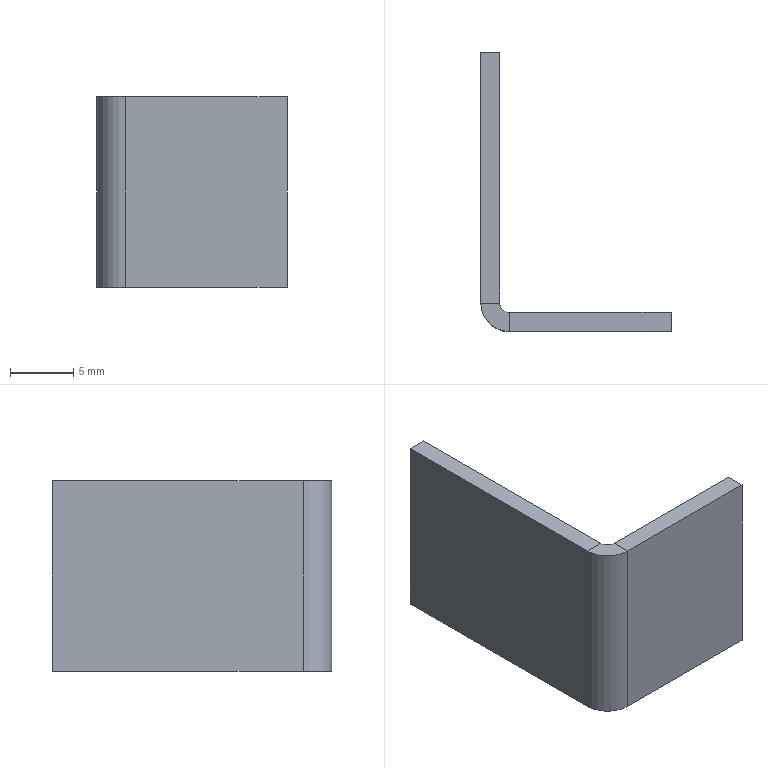Part | SolidWorks | features FlatPattern 1, SMBaseFlange 1, SheetMetal 1 | 1 solid | 14 faces | box 15 x 22 x 15 mm | volume 784.394 mm3 | plane 12 | cylinder 2 | commonest cylinder face diameters 1.473 x1 4.473 x1
STEP:
#1=CARTESIAN_POINT('',(-15.,2.237,7.5));
#2=VERTEX_POINT('',#1);
#3=CARTESIAN_POINT('',(-13.5,2.237,7.5));
#4=VERTEX_POINT('',#3);
#5=CARTESIAN_POINT('',(-15.,2.237,7.5));
#6=DIRECTION('',(1.,0.,0.));
#7=VECTOR('',#6,1000.);
#8=LINE('',#5,#7);
#9=EDGE_CURVE('',#2,#4,#8,.T.);
#10=ORIENTED_EDGE('',*,*,#9,.F.);
#11=CARTESIAN_POINT('',(-12.763,0.,7.5));
#12=VERTEX_POINT('',#11);
#13=CARTESIAN_POINT('',(-12.763,2.237,7.5));
#14=DIRECTION('',(0.,0.,-1.));
#15=DIRECTION('',(1.,0.,0.));
#16=AXIS2_PLACEMENT_3D('',#13,#14,#15);
#17=CIRCLE('',#16,2.237);
#18=EDGE_CURVE('',#12,#2,#17,.T.);
#19=ORIENTED_EDGE('',*,*,#18,.F.);
#20=CARTESIAN_POINT('',(-12.763,1.5,7.5));
#21=VERTEX_POINT('',#20);
#22=CARTESIAN_POINT('',(-12.763,1.5,7.5));
#23=DIRECTION('',(0.,-1.,0.));
#24=VECTOR('',#23,1000.);
#25=LINE('',#22,#24);
#26=EDGE_CURVE('',#21,#12,#25,.T.);
#27=ORIENTED_EDGE('',*,*,#26,.F.);
#28=CARTESIAN_POINT('',(-12.763,2.237,7.5));
#29=DIRECTION('',(0.,0.,-1.));
#30=DIRECTION('',(1.,0.,0.));
#31=AXIS2_PLACEMENT_3D('',#28,#29,#30);
#32=CIRCLE('',#31,0.7366);
#33=EDGE_CURVE('',#21,#4,#32,.T.);
#34=ORIENTED_EDGE('',*,*,#33,.T.);
#35=EDGE_LOOP('',(#10,#19,#27,#34));
#36=FACE_OUTER_BOUND('',#35,.T.);
#37=CARTESIAN_POINT('',(-15.,2.237,7.5));
#38=DIRECTION('',(0.,0.,1.));
#39=DIRECTION('',(1.,0.,0.));
#40=AXIS2_PLACEMENT_3D('',#37,#38,#39);
#41=PLANE('',#40);
#42=ADVANCED_FACE('',(#36),#41,.T.);
#43=CARTESIAN_POINT('',(-15.,22.,7.5));
#44=VERTEX_POINT('',#43);
#45=CARTESIAN_POINT('',(-15.,0.,7.5));
#46=DIRECTION('',(0.,1.,0.));
#47=VECTOR('',#46,1000.);
#48=LINE('',#45,#47);
#49=EDGE_CURVE('',#2,#44,#48,.T.);
#50=ORIENTED_EDGE('',*,*,#49,.F.);
#51=ORIENTED_EDGE('',*,*,#9,.T.);
#52=CARTESIAN_POINT('',(-13.5,22.,7.5));
#53=VERTEX_POINT('',#52);
#54=CARTESIAN_POINT('',(-13.5,0.,7.5));
#55=DIRECTION('',(0.,1.,0.));
#56=VECTOR('',#55,1000.);
#57=LINE('',#54,#56);
#58=EDGE_CURVE('',#4,#53,#57,.T.);
#59=ORIENTED_EDGE('',*,*,#58,.T.);
#60=CARTESIAN_POINT('',(-15.,22.,7.5));
#61=DIRECTION('',(1.,0.,0.));
#62=VECTOR('',#61,1000.);
#63=LINE('',#60,#62);
#64=EDGE_CURVE('',#44,#53,#63,.T.);
#65=ORIENTED_EDGE('',*,*,#64,.F.);
#66=EDGE_LOOP('',(#50,#51,#59,#65));
#67=FACE_OUTER_BOUND('',#66,.T.);
#68=CARTESIAN_POINT('',(-12.763,1.5,7.5));
#69=DIRECTION('',(0.,0.,1.));
#70=DIRECTION('',(1.,0.,0.));
#71=AXIS2_PLACEMENT_3D('',#68,#69,#70);
#72=PLANE('',#71);
#73=ADVANCED_FACE('',(#67),#72,.T.);
#74=CARTESIAN_POINT('',(-12.763,0.,-7.5));
#75=VERTEX_POINT('',#74);
#76=CARTESIAN_POINT('',(-12.763,1.5,-7.5));
#77=VERTEX_POINT('',#76);
#78=CARTESIAN_POINT('',(-12.763,0.,-7.5));
#79=DIRECTION('',(0.,1.,0.));
#80=VECTOR('',#79,1000.);
#81=LINE('',#78,#80);
#82=EDGE_CURVE('',#75,#77,#81,.T.);
#83=ORIENTED_EDGE('',*,*,#82,.F.);
#84=CARTESIAN_POINT('',(-15.,2.237,-7.5));
#85=VERTEX_POINT('',#84);
#86=CARTESIAN_POINT('',(-12.763,2.237,-7.5));
#87=DIRECTION('',(0.,0.,-1.));
#88=DIRECTION('',(1.,0.,0.));
#89=AXIS2_PLACEMENT_3D('',#86,#87,#88);
#90=CIRCLE('',#89,2.237);
#91=EDGE_CURVE('',#75,#85,#90,.T.);
#92=ORIENTED_EDGE('',*,*,#91,.T.);
#93=CARTESIAN_POINT('',(-13.5,2.237,-7.5));
#94=VERTEX_POINT('',#93);
#95=CARTESIAN_POINT('',(-13.5,2.237,-7.5));
#96=DIRECTION('',(-1.,0.,0.));
#97=VECTOR('',#96,1000.);
#98=LINE('',#95,#97);
#99=EDGE_CURVE('',#94,#85,#98,.T.);
#100=ORIENTED_EDGE('',*,*,#99,.F.);
#101=CARTESIAN_POINT('',(-12.763,2.237,-7.5));
#102=DIRECTION('',(0.,0.,-1.));
#103=DIRECTION('',(1.,0.,0.));
#104=AXIS2_PLACEMENT_3D('',#101,#102,#103);
#105=CIRCLE('',#104,0.7366);
#106=EDGE_CURVE('',#77,#94,#105,.T.);
#107=ORIENTED_EDGE('',*,*,#106,.F.);
#108=EDGE_LOOP('',(#83,#92,#100,#107));
#109=FACE_OUTER_BOUND('',#108,.T.);
#110=CARTESIAN_POINT('',(-12.763,0.,-7.5));
#111=DIRECTION('',(0.,0.,-1.));
#112=DIRECTION('',(-1.,0.,0.));
#113=AXIS2_PLACEMENT_3D('',#110,#111,#112);
#114=PLANE('',#113);
#115=ADVANCED_FACE('',(#109),#114,.T.);
#116=CARTESIAN_POINT('',(0.,0.,-7.5));
#117=VERTEX_POINT('',#116);
#118=CARTESIAN_POINT('',(0.,0.,-7.5));
#119=DIRECTION('',(-1.,0.,0.));
#120=VECTOR('',#119,1000.);
#121=LINE('',#118,#120);
#122=EDGE_CURVE('',#117,#75,#121,.T.);
#123=ORIENTED_EDGE('',*,*,#122,.T.);
#124=ORIENTED_EDGE('',*,*,#82,.T.);
#125=CARTESIAN_POINT('',(0.,1.5,-7.5));
#126=VERTEX_POINT('',#125);
#127=CARTESIAN_POINT('',(0.,1.5,-7.5));
#128=DIRECTION('',(-1.,0.,0.));
#129=VECTOR('',#128,1000.);
#130=LINE('',#127,#129);
#131=EDGE_CURVE('',#126,#77,#130,.T.);
#132=ORIENTED_EDGE('',*,*,#131,.F.);
#133=CARTESIAN_POINT('',(0.,1.5,-7.5));
#134=DIRECTION('',(0.,-1.,0.));
#135=VECTOR('',#134,1000.);
#136=LINE('',#133,#135);
#137=EDGE_CURVE('',#126,#117,#136,.T.);
#138=ORIENTED_EDGE('',*,*,#137,.T.);
#139=EDGE_LOOP('',(#123,#124,#132,#138));
#140=FACE_OUTER_BOUND('',#139,.T.);
#141=CARTESIAN_POINT('',(-13.5,2.237,-7.5));
#142=DIRECTION('',(0.,0.,-1.));
#143=DIRECTION('',(-1.,0.,0.));
#144=AXIS2_PLACEMENT_3D('',#141,#142,#143);
#145=PLANE('',#144);
#146=ADVANCED_FACE('',(#140),#145,.T.);
#147=CARTESIAN_POINT('',(-13.5,22.,-7.5));
#148=VERTEX_POINT('',#147);
#149=CARTESIAN_POINT('',(-13.5,0.,-7.5));
#150=DIRECTION('',(0.,1.,0.));
#151=VECTOR('',#150,1000.);
#152=LINE('',#149,#151);
#153=EDGE_CURVE('',#94,#148,#152,.T.);
#154=ORIENTED_EDGE('',*,*,#153,.T.);
#155=CARTESIAN_POINT('',(-13.5,22.,7.5));
#156=DIRECTION('',(0.,0.,-1.));
#157=VECTOR('',#156,1000.);
#158=LINE('',#155,#157);
#159=EDGE_CURVE('',#53,#148,#158,.T.);
#160=ORIENTED_EDGE('',*,*,#159,.F.);
#161=ORIENTED_EDGE('',*,*,#58,.F.);
#162=CARTESIAN_POINT('',(-13.5,2.237,7.5));
#163=DIRECTION('',(0.,0.,-1.));
#164=VECTOR('',#163,1000.);
#165=LINE('',#162,#164);
#166=EDGE_CURVE('',#4,#94,#165,.T.);
#167=ORIENTED_EDGE('',*,*,#166,.T.);
#168=EDGE_LOOP('',(#154,#160,#161,#167));
#169=FACE_OUTER_BOUND('',#168,.T.);
#170=CARTESIAN_POINT('',(-13.5,0.,7.5));
#171=DIRECTION('',(-1.,0.,0.));
#172=DIRECTION('',(0.,0.,1.));
#173=AXIS2_PLACEMENT_3D('',#170,#171,#172);
#174=PLANE('',#173);
#175=ADVANCED_FACE('',(#169),#174,.F.);
#176=CARTESIAN_POINT('',(-15.,22.,-7.5));
#177=VERTEX_POINT('',#176);
#178=CARTESIAN_POINT('',(-15.,22.,-7.5));
#179=DIRECTION('',(1.,0.,0.));
#180=VECTOR('',#179,1000.);
#181=LINE('',#178,#180);
#182=EDGE_CURVE('',#177,#148,#181,.T.);
#183=ORIENTED_EDGE('',*,*,#182,.F.);
#184=CARTESIAN_POINT('',(-15.,22.,7.5));
#185=DIRECTION('',(0.,0.,-1.));
#186=VECTOR('',#185,1000.);
#187=LINE('',#184,#186);
#188=EDGE_CURVE('',#44,#177,#187,.T.);
#189=ORIENTED_EDGE('',*,*,#188,.F.);
#190=ORIENTED_EDGE('',*,*,#64,.T.);
#191=ORIENTED_EDGE('',*,*,#159,.T.);
#192=EDGE_LOOP('',(#183,#189,#190,#191));
#193=FACE_OUTER_BOUND('',#192,.T.);
#194=CARTESIAN_POINT('',(-15.,22.,7.5));
#195=DIRECTION('',(0.,1.,0.));
#196=DIRECTION('',(0.,0.,1.));
#197=AXIS2_PLACEMENT_3D('',#194,#195,#196);
#198=PLANE('',#197);
#199=ADVANCED_FACE('',(#193),#198,.T.);
#200=CARTESIAN_POINT('',(-15.,0.,-7.5));
#201=DIRECTION('',(0.,1.,0.));
#202=VECTOR('',#201,1000.);
#203=LINE('',#200,#202);
#204=EDGE_CURVE('',#85,#177,#203,.T.);
#205=ORIENTED_EDGE('',*,*,#204,.F.);
#206=CARTESIAN_POINT('',(-15.,2.237,7.5));
#207=DIRECTION('',(0.,0.,-1.));
#208=VECTOR('',#207,1000.);
#209=LINE('',#206,#208);
#210=EDGE_CURVE('',#2,#85,#209,.T.);
#211=ORIENTED_EDGE('',*,*,#210,.F.);
#212=ORIENTED_EDGE('',*,*,#49,.T.);
#213=ORIENTED_EDGE('',*,*,#188,.T.);
#214=EDGE_LOOP('',(#205,#211,#212,#213));
#215=FACE_OUTER_BOUND('',#214,.T.);
#216=CARTESIAN_POINT('',(-15.,0.,7.5));
#217=DIRECTION('',(-1.,0.,0.));
#218=DIRECTION('',(0.,0.,1.));
#219=AXIS2_PLACEMENT_3D('',#216,#217,#218);
#220=PLANE('',#219);
#221=ADVANCED_FACE('',(#215),#220,.T.);
#222=ORIENTED_EDGE('',*,*,#91,.F.);
#223=CARTESIAN_POINT('',(-12.763,0.,7.5));
#224=DIRECTION('',(0.,0.,-1.));
#225=VECTOR('',#224,1000.);
#226=LINE('',#223,#225);
#227=EDGE_CURVE('',#12,#75,#226,.T.);
#228=ORIENTED_EDGE('',*,*,#227,.F.);
#229=ORIENTED_EDGE('',*,*,#18,.T.);
#230=ORIENTED_EDGE('',*,*,#210,.T.);
#231=EDGE_LOOP('',(#222,#228,#229,#230));
#232=FACE_OUTER_BOUND('',#231,.T.);
#233=CARTESIAN_POINT('',(-12.763,2.237,7.5));
#234=DIRECTION('',(0.,0.,-1.));
#235=DIRECTION('',(-1.,0.,0.));
#236=AXIS2_PLACEMENT_3D('',#233,#234,#235);
#237=CYLINDRICAL_SURFACE('',#236,2.237);
#238=ADVANCED_FACE('',(#232),#237,.T.);
#239=ORIENTED_EDGE('',*,*,#122,.F.);
#240=CARTESIAN_POINT('',(0.,0.,7.5));
#241=VERTEX_POINT('',#240);
#242=CARTESIAN_POINT('',(0.,0.,7.5));
#243=DIRECTION('',(0.,0.,-1.));
#244=VECTOR('',#243,1000.);
#245=LINE('',#242,#244);
#246=EDGE_CURVE('',#241,#117,#245,.T.);
#247=ORIENTED_EDGE('',*,*,#246,.F.);
#248=CARTESIAN_POINT('',(0.,0.,7.5));
#249=DIRECTION('',(-1.,0.,0.));
#250=VECTOR('',#249,1000.);
#251=LINE('',#248,#250);
#252=EDGE_CURVE('',#241,#12,#251,.T.);
#253=ORIENTED_EDGE('',*,*,#252,.T.);
#254=ORIENTED_EDGE('',*,*,#227,.T.);
#255=EDGE_LOOP('',(#239,#247,#253,#254));
#256=FACE_OUTER_BOUND('',#255,.T.);
#257=CARTESIAN_POINT('',(0.,0.,7.5));
#258=DIRECTION('',(0.,-1.,0.));
#259=DIRECTION('',(0.,0.,-1.));
#260=AXIS2_PLACEMENT_3D('',#257,#258,#259);
#261=PLANE('',#260);
#262=ADVANCED_FACE('',(#256),#261,.T.);
#263=ORIENTED_EDGE('',*,*,#137,.F.);
#264=CARTESIAN_POINT('',(0.,1.5,7.5));
#265=VERTEX_POINT('',#264);
#266=CARTESIAN_POINT('',(0.,1.5,7.5));
#267=DIRECTION('',(0.,0.,-1.));
#268=VECTOR('',#267,1000.);
#269=LINE('',#266,#268);
#270=EDGE_CURVE('',#265,#126,#269,.T.);
#271=ORIENTED_EDGE('',*,*,#270,.F.);
#272=CARTESIAN_POINT('',(0.,1.5,7.5));
#273=DIRECTION('',(0.,-1.,0.));
#274=VECTOR('',#273,1000.);
#275=LINE('',#272,#274);
#276=EDGE_CURVE('',#265,#241,#275,.T.);
#277=ORIENTED_EDGE('',*,*,#276,.T.);
#278=ORIENTED_EDGE('',*,*,#246,.T.);
#279=EDGE_LOOP('',(#263,#271,#277,#278));
#280=FACE_OUTER_BOUND('',#279,.T.);
#281=CARTESIAN_POINT('',(0.,1.5,7.5));
#282=DIRECTION('',(1.,0.,0.));
#283=DIRECTION('',(0.,0.,-1.));
#284=AXIS2_PLACEMENT_3D('',#281,#282,#283);
#285=PLANE('',#284);
#286=ADVANCED_FACE('',(#280),#285,.T.);
#287=ORIENTED_EDGE('',*,*,#131,.T.);
#288=CARTESIAN_POINT('',(-12.763,1.5,7.5));
#289=DIRECTION('',(0.,0.,-1.));
#290=VECTOR('',#289,1000.);
#291=LINE('',#288,#290);
#292=EDGE_CURVE('',#21,#77,#291,.T.);
#293=ORIENTED_EDGE('',*,*,#292,.F.);
#294=CARTESIAN_POINT('',(0.,1.5,7.5));
#295=DIRECTION('',(-1.,0.,0.));
#296=VECTOR('',#295,1000.);
#297=LINE('',#294,#296);
#298=EDGE_CURVE('',#265,#21,#297,.T.);
#299=ORIENTED_EDGE('',*,*,#298,.F.);
#300=ORIENTED_EDGE('',*,*,#270,.T.);
#301=EDGE_LOOP('',(#287,#293,#299,#300));
#302=FACE_OUTER_BOUND('',#301,.T.);
#303=CARTESIAN_POINT('',(0.,1.5,7.5));
#304=DIRECTION('',(0.,-1.,0.));
#305=DIRECTION('',(0.,0.,-1.));
#306=AXIS2_PLACEMENT_3D('',#303,#304,#305);
#307=PLANE('',#306);
#308=ADVANCED_FACE('',(#302),#307,.F.);
#309=ORIENTED_EDGE('',*,*,#106,.T.);
#310=ORIENTED_EDGE('',*,*,#166,.F.);
#311=ORIENTED_EDGE('',*,*,#33,.F.);
#312=ORIENTED_EDGE('',*,*,#292,.T.);
#313=EDGE_LOOP('',(#309,#310,#311,#312));
#314=FACE_OUTER_BOUND('',#313,.T.);
#315=CARTESIAN_POINT('',(-12.763,2.237,7.5));
#316=DIRECTION('',(0.,0.,-1.));
#317=DIRECTION('',(-1.,0.,0.));
#318=AXIS2_PLACEMENT_3D('',#315,#316,#317);
#319=CYLINDRICAL_SURFACE('',#318,0.7366);
#320=ADVANCED_FACE('',(#314),#319,.F.);
#321=ORIENTED_EDGE('',*,*,#298,.T.);
#322=ORIENTED_EDGE('',*,*,#26,.T.);
#323=ORIENTED_EDGE('',*,*,#252,.F.);
#324=ORIENTED_EDGE('',*,*,#276,.F.);
#325=EDGE_LOOP('',(#321,#322,#323,#324));
#326=FACE_OUTER_BOUND('',#325,.T.);
#327=CARTESIAN_POINT('',(-12.763,2.237,7.5));
#328=DIRECTION('',(0.,0.,1.));
#329=DIRECTION('',(1.,0.,0.));
#330=AXIS2_PLACEMENT_3D('',#327,#328,#329);
#331=PLANE('',#330);
#332=ADVANCED_FACE('',(#326),#331,.T.);
#333=ORIENTED_EDGE('',*,*,#153,.F.);
#334=ORIENTED_EDGE('',*,*,#99,.T.);
#335=ORIENTED_EDGE('',*,*,#204,.T.);
#336=ORIENTED_EDGE('',*,*,#182,.T.);
#337=EDGE_LOOP('',(#333,#334,#335,#336));
#338=FACE_OUTER_BOUND('',#337,.T.);
#339=CARTESIAN_POINT('',(-12.763,2.237,-7.5));
#340=DIRECTION('',(0.,0.,1.));
#341=DIRECTION('',(1.,0.,0.));
#342=AXIS2_PLACEMENT_3D('',#339,#340,#341);
#343=PLANE('',#342);
#344=ADVANCED_FACE('',(#338),#343,.F.);
#345=CLOSED_SHELL('',(#42,#73,#115,#146,#175,#199,#221,#238,#262,#286,#308,#320,#332,#344));
#346=MANIFOLD_SOLID_BREP('',#345);
#347=CARTESIAN_POINT('',(0.,0.,0.));
#348=DIRECTION('',(0.,0.,1.));
#349=DIRECTION('',(1.,0.,0.));
#350=AXIS2_PLACEMENT_3D('',#347,#348,#349);
#351=(LENGTH_UNIT()NAMED_UNIT(*)SI_UNIT(.MILLI.,.METRE.));
#352=UNCERTAINTY_MEASURE_WITH_UNIT(LENGTH_MEASURE(0.00001),#351,'','');
#353=(NAMED_UNIT(*)PLANE_ANGLE_UNIT()SI_UNIT($,.RADIAN.));
#354=(NAMED_UNIT(*)SI_UNIT($,.STERADIAN.)SOLID_ANGLE_UNIT());
#355=(GEOMETRIC_REPRESENTATION_CONTEXT(3)GLOBAL_UNCERTAINTY_ASSIGNED_CONTEXT((#352))GLOBAL_UNIT_ASSIGNED_CONTEXT((#351,#353,#354))REPRESENTATION_CONTEXT('',''));
#356=ADVANCED_BREP_SHAPE_REPRESENTATION('',(#346,#350),#355);